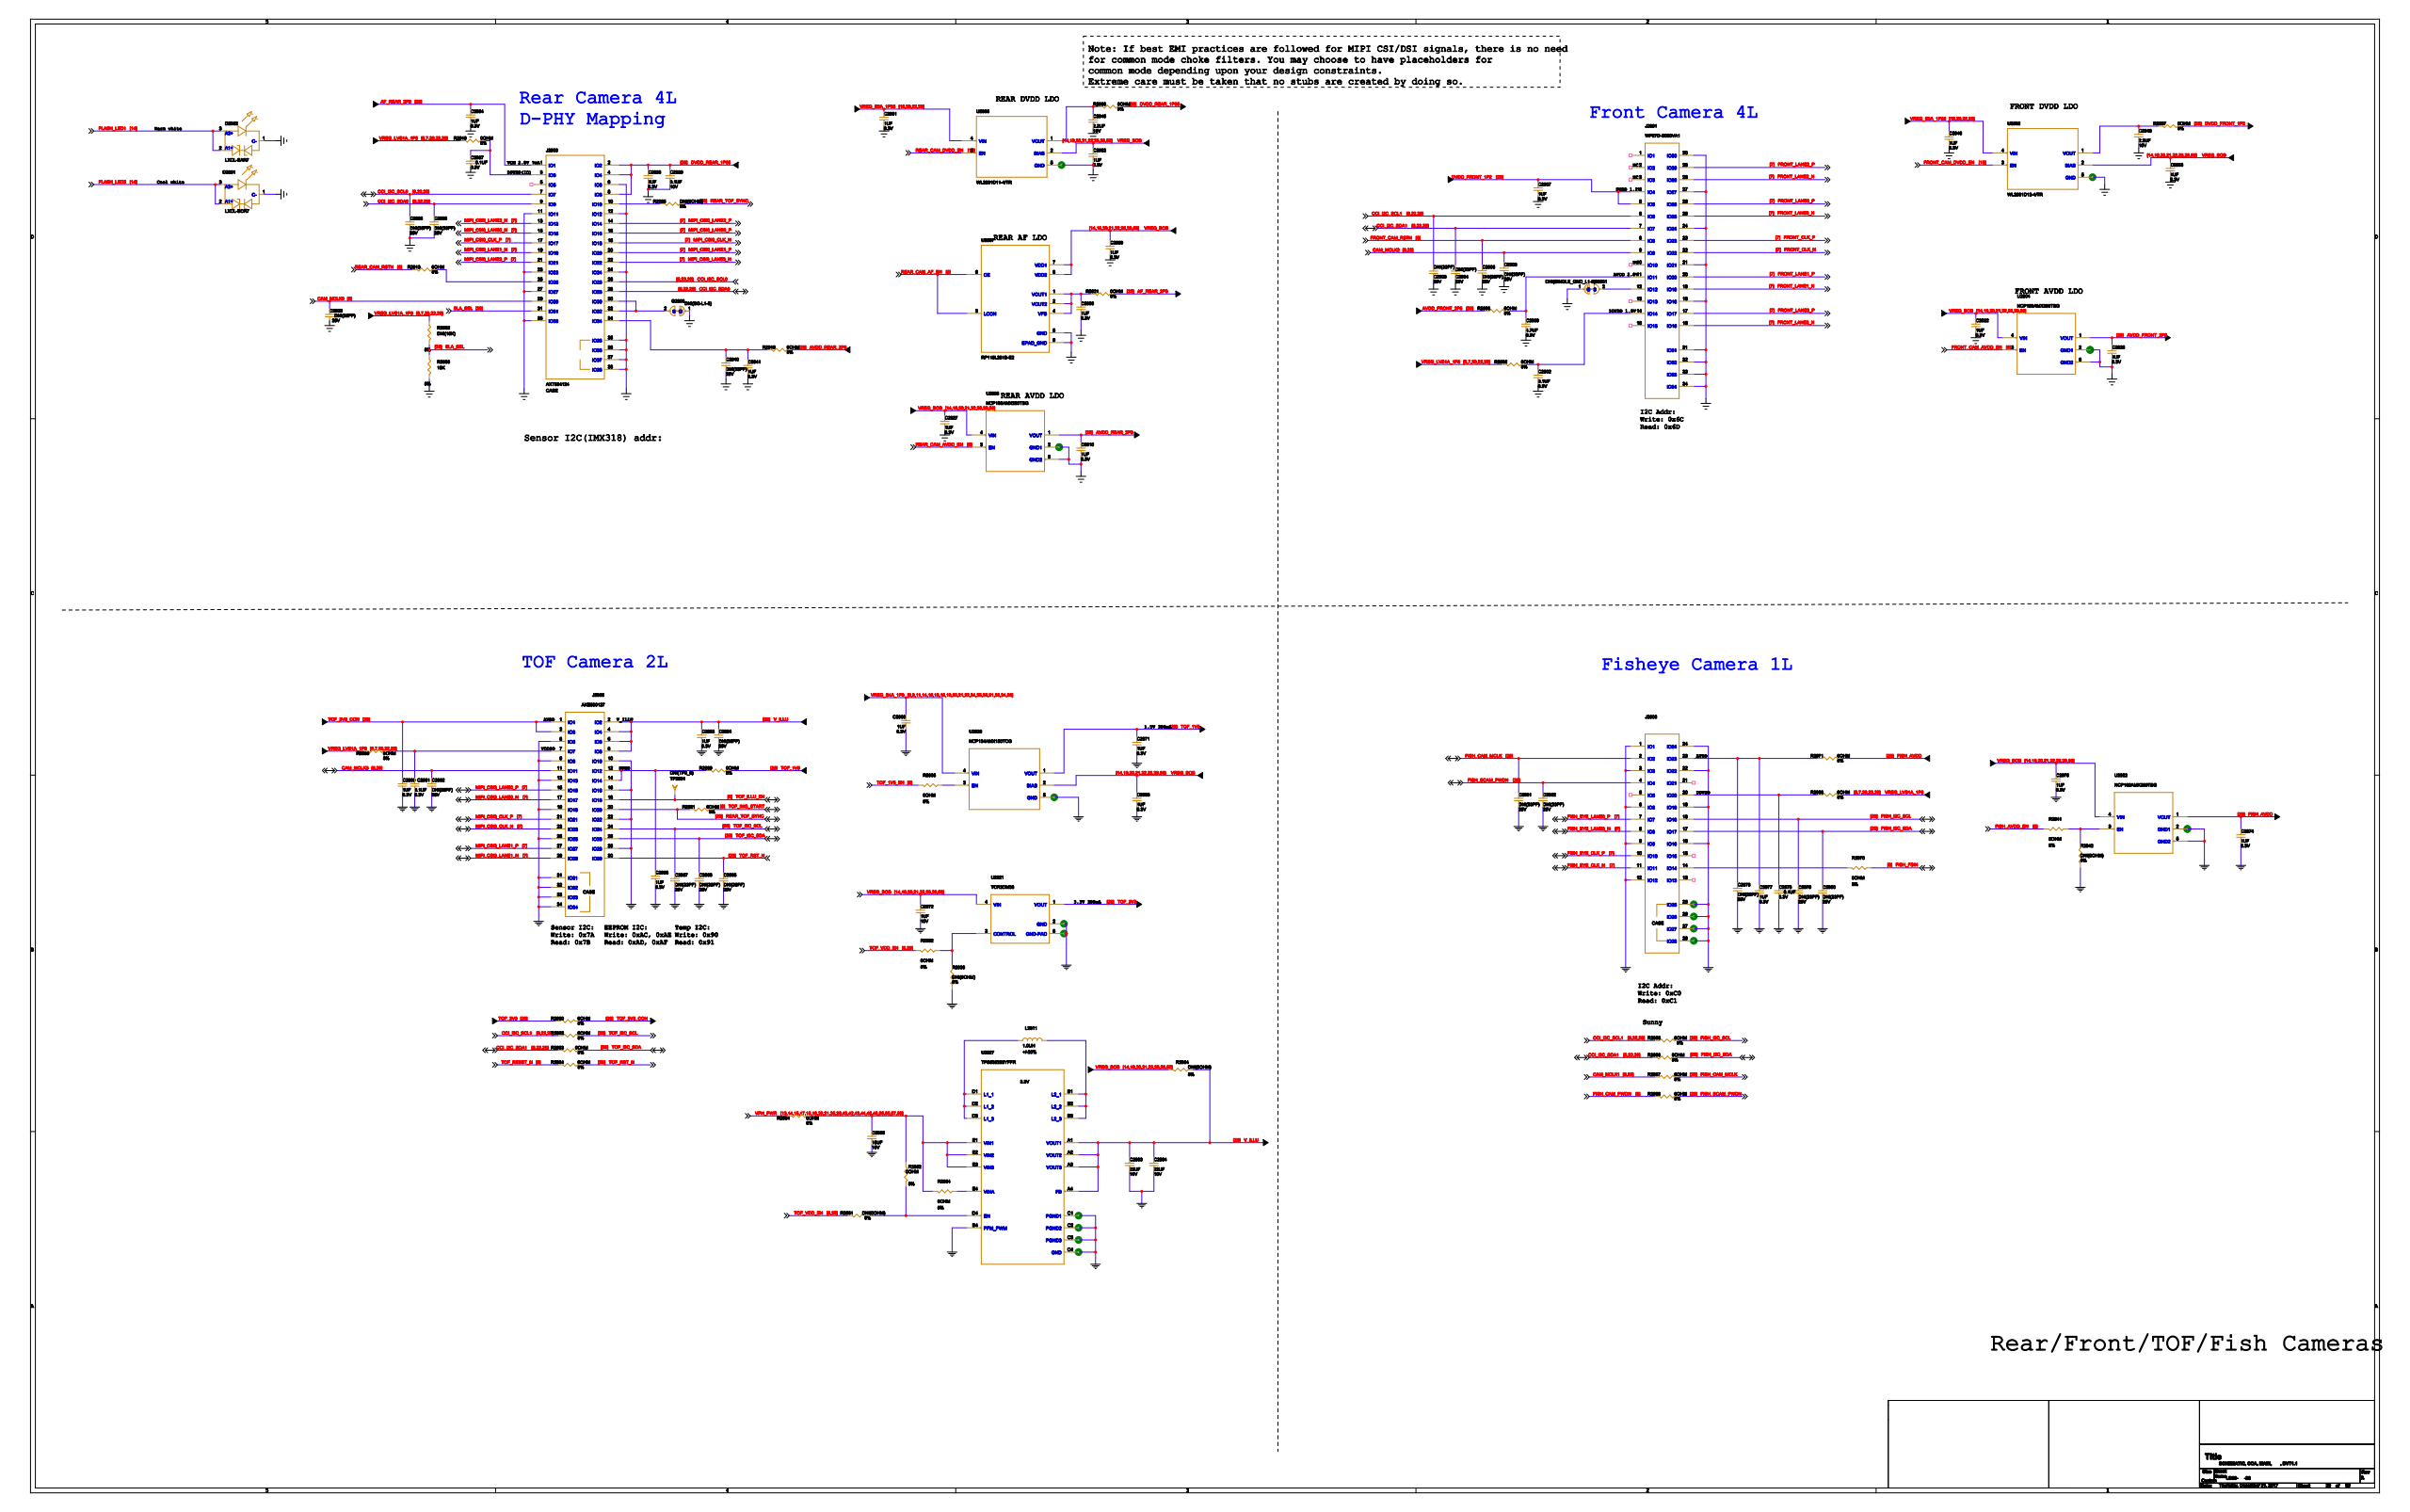Circuit board | Cadence Allegro | 1520 parts | 1149 nets | one sheet of the schematic
Parts on this sheet (reference | value | footprint):
C2902 | 0.1UF | 2P0201R
C2903 | DNI(33PF) | 2P0201R_DNI
C2904 | DNI(33PF) | 2P0201R_DNI
C2905 | DNI(33PF) | 2P0201R_DNI
C2907 | 1UF | 2P0201R
C2909 | 4.7UF | 2P0603R
C2910 | 1UF | 2P0201R
C2922 | 1UF | 2P0201R
C2926 | 1UF | 2P0201R
C2927 | 1UF | 2P0201R
C2929 | DNI(33PF) | 2P0201R_DNI
C2934 | 1UF | 2P0201R
C2935 | DNI(33PF) | 2P0201R_DNI
C2936 | DNI(33PF) | 2P0201R_DNI
C2937 | 0.1UF | 2P0201R
C2938 | 1UF | 2P0201R
C2939 | 0.1UF | 2P0201R
C2940 | DNI(33PF) | 2P0201R_DNI
C2941 | 1UF | 2P0201R
C2945 | 2.2UF | 2P0201R
C2946 | 1UF | 2P0201R
C2948 | 2.2UF | 2P0201R
C2951 | 1UF | 2P0201R
C2952 | 1UF | 2P0201R
C2953 | 1UF | 2P0201R
C2956 | 1UF | 2P0201R
C2959 | 1UF | 2P0201R
C2960 | 1UF | 2P0201R
C2961 | 0.1UF | 2P0201R
C2962 | DNI(33PF) | 2P0201R_DNI
C2963 | 1UF | 2P0201R
C2964 | DNI(33PF) | 2P0201R_DNI
C2965 | DNI(33PF) | 2P0201R_DNI
C2966 | DNI(33PF) | 2P0201R_DNI
C2967 | DNI(33PF) | 2P0201R_DNI
C2969 | 1UF | 2P0201R
C2971 | 1UF | 2P0201R
C2972 | 1UF | 2P0402R
C2974 | 1UF | 2P0201R
C2975 | 1UF | 2P0201R
C2976 | DNI(33PF) | 2P0201R_DNI
C2977 | 1UF | 2P0201R
C2978 | 0.1UF | 2P0201R
C2979 | DNI(33PF) | 2P0201R_DNI
C2980 | DNI(33PF) | 2P0201R_DNI
C2981 | DNI(33PF) | 2P0201R_DNI
C2982 | DNI(33PF) | 2P0201R_DNI
C2983 | 22UF | 2P0603R
C2984 | 22UF | 2P0603R
C2985 | 10UF | 2P0603R
C2986 | 1UF | 2P0201R
D2901 | LXCL-ECR7 | 3PSM84X69N
D2902 | LXCL-EAR7 | 3PSM84X69N
G2901 | DNI(SINGLE_GND_L1-5) | GND_L1-5
J2901 | WP27D-S030VA1 | 34SCONS138V3_CCW
J2903 | AXT534124 | 38SCONS157V8
J2905 | AXE530127 | 34SCONS157V7
J2906 | AXE524127 | 28SCONS157V7_CW
L2911 | 1.0UH | 2PSM87X71NV2
R2902 | 0OHM | 2P0201R
R2903 | 0OHM | 2P0201R
R2910 | 0OHM | 2P0201R
R2913 | 0OHM | 2P0201R
R2916 | 0OHM | 2P0201R
R2921 | 0OHM | 2P0201R
R2932 | 0OHM | 2P0201R
R2933 | DNI(0OHM) | 2P0201R_DNI
R2935 | 0OHM | 2P0201R
R2941 | 0OHM | 2P0201R
R2942 | DNI(0OHM) | 2P0201R_DNI
R2951 | DNI(0OHM) | 2P0201R_DNI
R2952 | 0OHM | 2P0201R
R2954 | 0OHM | 2P0201R
R2960 | 0OHM | 2P0201R
R2961 | 0OHM | 2P0603R
R2962 | 0OHM | 2P0201R
R2963 | 0OHM | 2P0201R
R2964 | 0OHM | 2P0201R
R2965 | 0OHM | 2P0201R
R2966 | 0OHM | 2P0201R
R2967 | 0OHM | 2P0201R
R2968 | 0OHM | 2P0201R
R2970 | 0OHM | 2P0201R
R2971 | 0OHM | 2P0201R
R2980 | 0OHM | 2P0201R
R2981 | 0OHM | 2P0201R
R2982 | DNI(10K) | 2P0201R_DNI
R2983 | 10K | 2P0201R
R2984 | DNI(0OHM) | 2P0603R_DNI
R2985 | DNI(0OHM) | 2P0201R_DNI
R2986 | 0OHM | 2P0201R
R2987 | 0OHM | 2P0201R
R2988 | 0OHM | 2P0201R
R2989 | 0OHM | 2P0201R
TP2901 | DNI(TP0_6) | TP-0_6
U2902 | WL2831D12-4/TR | 5PSM49X49N
U2904 | NCP160AMX280TBG | 5PSM39X39N
U2905 | NCP160AMX280TBG | 5PSM39X39N
U2906 | WL2831D11-4/TR | 5PSM49X49N
U2907 | RP115L281B-E2 | 9PSM65X49N157
U2920 | NCP134AMX150TCG | 5PSM49X49N
U2921 | TCR3DM33 | 5PSM41X41NV1
U2922 | NCP160AMX280TBG | 5PSM39X39N
U2927 | TPS630252YFFR | 20PGA83X71B157
Nets of these parts (net: part-pin ...):
GND: C2902-2 C2903-1 C2904-1 C2905-2 C2907-2 C2909-2 C2910-2 C2922-2 C2926-2 C2927-2 C2929-2 C2934-2 C2935-2 C2936-2 C2937-2 C2938-2 C2939-2 C2940-2 C2941-2 C2945-2 C2946-2 C2948-2 C2951-2 C2952-2 C2953-2 C2956-2 C2959-2 C2960-2 C2961-2 C2962-2 C2963-2 C2964-2 C2965-2 C2966-2 C2967-2 C2969-2 C2971-2 C2972-2 C2974-2 C2975-2 C2976-2 C2977-2 C2978-2 C2979-2 C2980-2 C2981-2 C2982-2 C2983-2 C2984-2 C2985-2 C2986-2 D2901-1 D2902-1 G2901-1 R2933-2 R2942-2 R2983-1 U2902-5 U2904-2 U2904-5 U2905-2 U2905-5 U2906-5 U2907-5 U2907-9 U2920-5 U2921-2 U2921-5 U2922-2 U2922-5 U2927-B4 U2927-C1 U2927-C2 U2927-C3 U2927-C4 J2901-18 J2901-21 J2901-24 J2901-27 J2901-30 J2901-31 J2901-32 J2901-33 J2901-34 J2903-6 J2903-11 J2903-12 J2903-23 J2903-24 J2903-27 J2903-33 J2903-35 J2903-36 J2903-37 J2903-38 J2905-5 J2905-9 J2905-10 J2905-13 J2905-16 J2905-19 J2905-22 J2905-25 J2905-28 J2905-31 J2905-32 J2905-33 J2905-34 J2906-1 J2906-3 J2906-6 J2906-9 J2906-12 J2906-16 J2906-19 J2906-22 J2906-24 J2906-25 J2906-26 J2906-27 J2906-28
VREG_BOB: C2922-1 C2927-1 C2952-1 C2953-1 C2959-1 C2972-1 C2975-1 C2986-1 R2984-1 U2902-2 U2904-4 U2905-4 U2906-2 U2907-7 U2907-8 U2920-2 U2921-4 U2922-4
N52256871: R2935-2 U2920-3
VREG_S4A_1P8: C2969-1 U2920-4
TOF_1V5: C2971-1 R2980-2 U2920-1
FLASH_LED2: D2901-2 D2901-3
FLASH_LED1: D2902-2 D2902-3
N34857651: G2901-2 J2901-12
VPH_PWR: R2961-1
CCI_I2C_SCL1: C2903-2 R2962-2 R2965-2 J2901-6
CCI_I2C_SDA1: C2904-2 R2963-1 R2966-1 J2901-7
CAM_MCLK2: J2901-9
VREG_S3A_1P35: C2946-1 C2951-1 U2902-4 U2906-4
VREG_LVS1A_1P8: R2902-1 R2910-1 R2982-2 R2988-1 R2989-1
CAM_MCLK1: R2967-2
CCI_I2C_SDA0: C2936-1 J2903-9 J2903-28
CCI_I2C_SCL0: C2935-1 J2903-7 J2903-26
REAR_CAM_DVDD_EN: U2906-3
N48961365: C2945-1 R2986-1 U2906-1
AF_REAR_2P8: C2934-1 R2921-2 J2903-1
N49759744: R2985-1 J2903-10
MIPI_CSI0_LANE2_N: J2903-13
MIPI_CSI0_LANE2_P: J2903-14
MIPI_CSI0_LANE0_N: J2903-15
MIPI_CSI0_LANE0_P: J2903-16
MIPI_CSI0_CLK_P: J2903-17
MIPI_CSI0_CLK_N: J2903-18
MIPI_CSI0_LANE1_N: J2903-19
DVDD_REAR_1P05: C2938-1 C2939-1 R2986-2 J2903-2 J2903-4 J2903-8
MIPI_CSI0_LANE1_P: J2903-20
MIPI_CSI0_LANE3_P: J2903-21
MIPI_CSI0_LANE3_N: J2903-22
N48884852: R2913-2 J2903-25
CAM_MCLK0: C2929-1 J2903-29
N48879197: C2937-1 R2910-2 J2903-3
SLA_SEL: R2982-1 R2983-2 J2903-31
N35055984: C2940-1 C2941-1 R2916-1 J2903-34
V_ILLU: C2963-1 C2964-1 C2983-1 C2984-1 R2984-2 U2927-A1 U2927-A2 U2927-A3 U2927-A4 J2905-2 J2905-4 J2905-6 J2905-8
FRONT_CAM_DVDD_EN: U2902-3
N35065811: C2948-1 R2987-1 U2902-1
FRONT_CAM_AVDD_EN: U2904-3
AVDD_FRONT_2P8: C2926-1 R2903-1 U2904-1
REAR_CAM_AVDD_EN: U2905-3
AVDD_REAR_2P8: C2910-1 R2916-2 U2905-1
N49636672: R2941-2 R2942-1 U2922-3
FISH_AVDD: C2974-1 R2971-1 U2922-1
REAR_CAM_AF_EN: U2907-3 U2907-6
N37904999: C2956-1 R2921-1 U2907-1 U2907-2 U2907-4
FRONT_CLK_N: J2901-22
FRONT_CLK_P: J2901-23
FRONT_LANE0_N: J2901-25
FRONT_LANE0_P: J2901-26
FRONT_LANE1_N: J2901-19
FRONT_LANE1_P: J2901-20
FRONT_LANE2_N: J2901-28
FRONT_LANE2_P: J2901-29
FRONT_LANE3_N: J2901-16
FRONT_LANE3_P: J2901-17
CAM_MCLK3: C2962-1 J2905-11
N34857817: C2902-1 R2902-2 J2901-14
N49636387: C2961-1 R2989-2 J2905-7
N49635812: C2978-1 R2988-2 J2906-20
DVDD_FRONT_1P2: C2907-1 R2987-2 J2901-4 J2901-5
TOF_3V3_CON: C2960-1 R2960-1 J2905-1 J2905-3
N49636321: R2980-1 J2905-12 J2905-14
N49635910: C2976-1 C2977-1 R2971-2 J2906-23
FRONT_CAM_RSTN: C2905-1 J2901-8
TOF_RST_N: C2965-1 R2964-2 J2905-30
TOF_I2C_SDA: C2966-1 R2963-2 J2905-26
TOF_I2C_SCL: C2967-1 R2962-1 J2905-24
FISH_I2C_SCL: C2979-1 R2965-1 J2906-18
FISH_I2C_SDA: C2980-1 R2966-2 J2906-17
FISH_CAM_MCLK: C2981-1 R2967-1 J2906-2
FISH_SCAM_PWDN: C2982-1 R2968-2 J2906-4
N34857752: C2909-1 R2903-2 J2901-11
N49635992: C2985-1 R2952-2 R2954-1 R2961-2 U2927-E1 U2927-E2 U2927-E3
TOF_RESET_N: R2964-1
FISH_CAM_PWDN: R2968-1
REAR_TOF_SYNC: R2981-1 R2985-2 J2905-20
TOF_IMG_START: R2981-2
REAR_CAM_RSTN: R2913-1
TOF_VDD_EN: R2932-1 R2951-1
N49637008: R2932-2 R2933-1 U2921-3
TOF_1V5_EN: R2935-1
FISH_AVDD_EN: R2941-1
N49636064: R2951-2 R2952-1 U2927-D4
N49636046: R2954-2 U2927-E4
TOF_3V3: R2960-2 U2921-1
N49637313: R2970-1 J2906-14
FISH_FSIN: R2970-2
FISH_EYE_CLK_P: J2906-10
FISH_EYE_CLK_N: J2906-11
FISH_EYE_LANE0_P: J2906-7
FISH_EYE_LANE0_N: J2906-8
MIPI_CSI3_LANE0_P: J2905-15
MIPI_CSI3_LANE0_N: J2905-17
TOF_ILLU_EN: TP2901-1 J2905-18
MIPI_CSI3_CLK_P: J2905-21
MIPI_CSI3_CLK_N: J2905-23
MIPI_CSI3_LANE1_P: J2905-27
MIPI_CSI3_LANE1_N: J2905-29
N49636104: L2911-1 U2927-D1 U2927-D2 U2927-D3
N49636090: L2911-2 U2927-B1 U2927-B2 U2927-B3